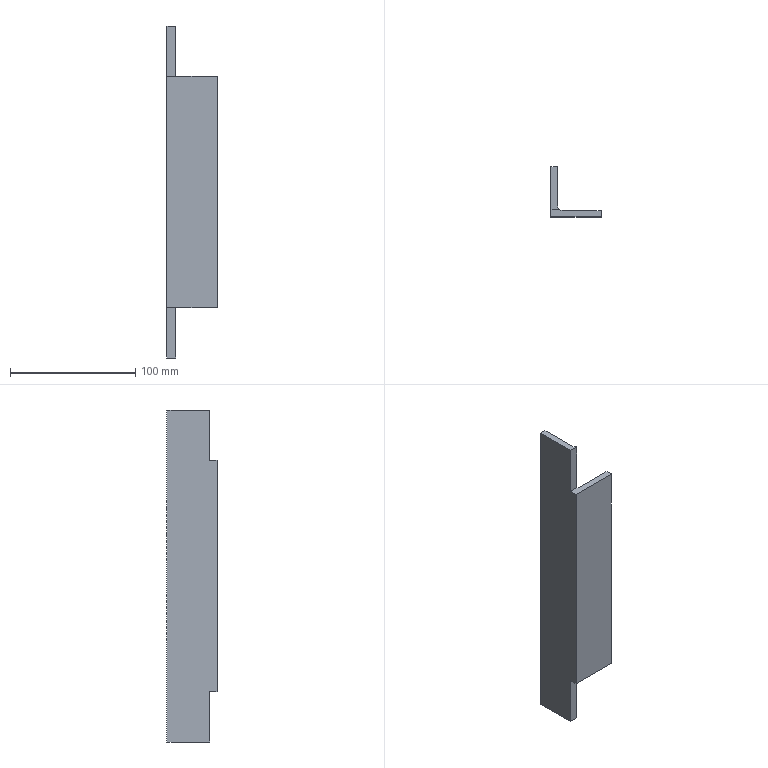Part | NX | features BREP 1 | 1 solid | 13 faces | box 40 x 40 x 265 mm | volume 84160 mm3 | plane 12 | cylinder 1 | commonest cylinder face diameters 10 x1
STEP:
#1=CARTESIAN_POINT('',(40.,5.,92.5));
#2=VERTEX_POINT('',#1);
#3=CARTESIAN_POINT('',(40.,5.,-92.5));
#4=VERTEX_POINT('',#3);
#5=CARTESIAN_POINT('',(40.,5.,132.5));
#6=DIRECTION('',(0.,0.,-1.));
#7=VECTOR('',#6,1000.);
#8=LINE('',#5,#7);
#9=EDGE_CURVE('',#2,#4,#8,.T.);
#10=ORIENTED_EDGE('',*,*,#9,.F.);
#11=CARTESIAN_POINT('',(40.,0.,92.5));
#12=VERTEX_POINT('',#11);
#13=CARTESIAN_POINT('',(40.,0.,92.5));
#14=DIRECTION('',(0.,-1.,0.));
#15=VECTOR('',#14,1000.);
#16=LINE('',#13,#15);
#17=EDGE_CURVE('',#2,#12,#16,.T.);
#18=ORIENTED_EDGE('',*,*,#17,.T.);
#19=CARTESIAN_POINT('',(40.,0.,-92.5));
#20=VERTEX_POINT('',#19);
#21=CARTESIAN_POINT('',(40.,0.,132.5));
#22=DIRECTION('',(0.,0.,-1.));
#23=VECTOR('',#22,1000.);
#24=LINE('',#21,#23);
#25=EDGE_CURVE('',#12,#20,#24,.T.);
#26=ORIENTED_EDGE('',*,*,#25,.T.);
#27=CARTESIAN_POINT('',(40.,0.,-92.5));
#28=DIRECTION('',(0.,1.,0.));
#29=VECTOR('',#28,1000.);
#30=LINE('',#27,#29);
#31=EDGE_CURVE('',#20,#4,#30,.T.);
#32=ORIENTED_EDGE('',*,*,#31,.T.);
#33=EDGE_LOOP('',(#10,#18,#26,#32));
#34=FACE_BOUND('',#33,.T.);
#35=CARTESIAN_POINT('',(40.,5.,132.5));
#36=DIRECTION('',(-1.,0.,0.));
#37=DIRECTION('',(0.,0.,-1.));
#38=AXIS2_PLACEMENT_3D('',#35,#36,#37);
#39=PLANE('',#38);
#40=ADVANCED_FACE('',(#34),#39,.F.);
#41=CARTESIAN_POINT('',(10.,5.,92.5));
#42=VERTEX_POINT('',#41);
#43=CARTESIAN_POINT('',(10.,5.,-92.5));
#44=VERTEX_POINT('',#43);
#45=CARTESIAN_POINT('',(10.,5.,132.5));
#46=DIRECTION('',(0.,0.,-1.));
#47=VECTOR('',#46,1000.);
#48=LINE('',#45,#47);
#49=EDGE_CURVE('',#42,#44,#48,.T.);
#50=ORIENTED_EDGE('',*,*,#49,.F.);
#51=CARTESIAN_POINT('',(10.,5.,92.5));
#52=DIRECTION('',(1.,0.,0.));
#53=VECTOR('',#52,1000.);
#54=LINE('',#51,#53);
#55=EDGE_CURVE('',#42,#2,#54,.T.);
#56=ORIENTED_EDGE('',*,*,#55,.T.);
#57=ORIENTED_EDGE('',*,*,#9,.T.);
#58=CARTESIAN_POINT('',(10.,5.,-92.5));
#59=DIRECTION('',(-1.,0.,0.));
#60=VECTOR('',#59,1000.);
#61=LINE('',#58,#60);
#62=EDGE_CURVE('',#4,#44,#61,.T.);
#63=ORIENTED_EDGE('',*,*,#62,.T.);
#64=EDGE_LOOP('',(#50,#56,#57,#63));
#65=FACE_BOUND('',#64,.T.);
#66=CARTESIAN_POINT('',(10.,5.,132.5));
#67=DIRECTION('',(0.,-1.,0.));
#68=DIRECTION('',(0.,0.,1.));
#69=AXIS2_PLACEMENT_3D('',#66,#67,#68);
#70=PLANE('',#69);
#71=ADVANCED_FACE('',(#65),#70,.F.);
#72=CARTESIAN_POINT('',(7.,6.,132.5));
#73=VERTEX_POINT('',#72);
#74=CARTESIAN_POINT('',(7.,6.,92.5));
#75=VERTEX_POINT('',#74);
#76=CARTESIAN_POINT('',(7.,6.,132.5));
#77=DIRECTION('',(0.,0.,-1.));
#78=VECTOR('',#77,1000.);
#79=LINE('',#76,#78);
#80=EDGE_CURVE('',#73,#75,#79,.T.);
#81=ORIENTED_EDGE('',*,*,#80,.T.);
#82=CARTESIAN_POINT('',(10.,10.,92.5));
#83=DIRECTION('',(0.,0.,1.));
#84=DIRECTION('',(-1.,0.,0.));
#85=AXIS2_PLACEMENT_3D('',#82,#83,#84);
#86=CIRCLE('',#85,5.);
#87=EDGE_CURVE('',#75,#42,#86,.T.);
#88=ORIENTED_EDGE('',*,*,#87,.T.);
#89=ORIENTED_EDGE('',*,*,#49,.T.);
#90=CARTESIAN_POINT('',(7.,6.,-92.5));
#91=VERTEX_POINT('',#90);
#92=CARTESIAN_POINT('',(10.,10.,-92.5));
#93=DIRECTION('',(0.,0.,-1.));
#94=DIRECTION('',(1.,0.,0.));
#95=AXIS2_PLACEMENT_3D('',#92,#93,#94);
#96=CIRCLE('',#95,5.);
#97=EDGE_CURVE('',#44,#91,#96,.T.);
#98=ORIENTED_EDGE('',*,*,#97,.T.);
#99=CARTESIAN_POINT('',(7.,6.,-132.5));
#100=VERTEX_POINT('',#99);
#101=CARTESIAN_POINT('',(7.,6.,132.5));
#102=DIRECTION('',(0.,0.,-1.));
#103=VECTOR('',#102,1000.);
#104=LINE('',#101,#103);
#105=EDGE_CURVE('',#91,#100,#104,.T.);
#106=ORIENTED_EDGE('',*,*,#105,.T.);
#107=CARTESIAN_POINT('',(5.,10.,-132.5));
#108=VERTEX_POINT('',#107);
#109=CARTESIAN_POINT('',(10.,10.,-132.5));
#110=DIRECTION('',(0.,0.,-1.));
#111=DIRECTION('',(1.,0.,0.));
#112=AXIS2_PLACEMENT_3D('',#109,#110,#111);
#113=CIRCLE('',#112,5.);
#114=EDGE_CURVE('',#100,#108,#113,.T.);
#115=ORIENTED_EDGE('',*,*,#114,.T.);
#116=CARTESIAN_POINT('',(5.,10.,132.5));
#117=VERTEX_POINT('',#116);
#118=CARTESIAN_POINT('',(5.,10.,132.5));
#119=DIRECTION('',(0.,0.,-1.));
#120=VECTOR('',#119,1000.);
#121=LINE('',#118,#120);
#122=EDGE_CURVE('',#117,#108,#121,.T.);
#123=ORIENTED_EDGE('',*,*,#122,.F.);
#124=CARTESIAN_POINT('',(10.,10.,132.5));
#125=DIRECTION('',(0.,0.,-1.));
#126=DIRECTION('',(1.,0.,0.));
#127=AXIS2_PLACEMENT_3D('',#124,#125,#126);
#128=CIRCLE('',#127,5.);
#129=EDGE_CURVE('',#73,#117,#128,.T.);
#130=ORIENTED_EDGE('',*,*,#129,.F.);
#131=EDGE_LOOP('',(#81,#88,#89,#98,#106,#115,#123,#130));
#132=FACE_BOUND('',#131,.T.);
#133=CARTESIAN_POINT('',(10.,10.,132.5));
#134=DIRECTION('',(0.,0.,-1.));
#135=DIRECTION('',(1.,0.,0.));
#136=AXIS2_PLACEMENT_3D('',#133,#134,#135);
#137=CYLINDRICAL_SURFACE('',#136,5.);
#138=ADVANCED_FACE('',(#132),#137,.F.);
#139=CARTESIAN_POINT('',(5.,40.,-132.5));
#140=VERTEX_POINT('',#139);
#141=CARTESIAN_POINT('',(5.,40.,-132.5));
#142=DIRECTION('',(0.,1.,0.));
#143=VECTOR('',#142,1000.);
#144=LINE('',#141,#143);
#145=EDGE_CURVE('',#108,#140,#144,.T.);
#146=ORIENTED_EDGE('',*,*,#145,.T.);
#147=CARTESIAN_POINT('',(5.,40.,132.5));
#148=VERTEX_POINT('',#147);
#149=CARTESIAN_POINT('',(5.,40.,132.5));
#150=DIRECTION('',(0.,0.,-1.));
#151=VECTOR('',#150,1000.);
#152=LINE('',#149,#151);
#153=EDGE_CURVE('',#148,#140,#152,.T.);
#154=ORIENTED_EDGE('',*,*,#153,.F.);
#155=CARTESIAN_POINT('',(5.,40.,132.5));
#156=DIRECTION('',(0.,1.,0.));
#157=VECTOR('',#156,1000.);
#158=LINE('',#155,#157);
#159=EDGE_CURVE('',#117,#148,#158,.T.);
#160=ORIENTED_EDGE('',*,*,#159,.F.);
#161=ORIENTED_EDGE('',*,*,#122,.T.);
#162=EDGE_LOOP('',(#146,#154,#160,#161));
#163=FACE_BOUND('',#162,.T.);
#164=CARTESIAN_POINT('',(5.,40.,132.5));
#165=DIRECTION('',(-1.,0.,0.));
#166=DIRECTION('',(0.,0.,-1.));
#167=AXIS2_PLACEMENT_3D('',#164,#165,#166);
#168=PLANE('',#167);
#169=ADVANCED_FACE('',(#163),#168,.F.);
#170=CARTESIAN_POINT('',(0.,40.,-132.5));
#171=VERTEX_POINT('',#170);
#172=CARTESIAN_POINT('',(0.,40.,-132.5));
#173=DIRECTION('',(-1.,0.,0.));
#174=VECTOR('',#173,1000.);
#175=LINE('',#172,#174);
#176=EDGE_CURVE('',#140,#171,#175,.T.);
#177=ORIENTED_EDGE('',*,*,#176,.T.);
#178=CARTESIAN_POINT('',(0.,40.,132.5));
#179=VERTEX_POINT('',#178);
#180=CARTESIAN_POINT('',(0.,40.,132.5));
#181=DIRECTION('',(0.,0.,-1.));
#182=VECTOR('',#181,1000.);
#183=LINE('',#180,#182);
#184=EDGE_CURVE('',#179,#171,#183,.T.);
#185=ORIENTED_EDGE('',*,*,#184,.F.);
#186=CARTESIAN_POINT('',(0.,40.,132.5));
#187=DIRECTION('',(-1.,0.,0.));
#188=VECTOR('',#187,1000.);
#189=LINE('',#186,#188);
#190=EDGE_CURVE('',#148,#179,#189,.T.);
#191=ORIENTED_EDGE('',*,*,#190,.F.);
#192=ORIENTED_EDGE('',*,*,#153,.T.);
#193=EDGE_LOOP('',(#177,#185,#191,#192));
#194=FACE_BOUND('',#193,.T.);
#195=CARTESIAN_POINT('',(0.,40.,132.5));
#196=DIRECTION('',(0.,-1.,0.));
#197=DIRECTION('',(0.,0.,1.));
#198=AXIS2_PLACEMENT_3D('',#195,#196,#197);
#199=PLANE('',#198);
#200=ADVANCED_FACE('',(#194),#199,.F.);
#201=CARTESIAN_POINT('',(0.,0.,92.5));
#202=VERTEX_POINT('',#201);
#203=CARTESIAN_POINT('',(0.,0.,-92.5));
#204=VERTEX_POINT('',#203);
#205=CARTESIAN_POINT('',(0.,0.,132.5));
#206=DIRECTION('',(0.,0.,-1.));
#207=VECTOR('',#206,1000.);
#208=LINE('',#205,#207);
#209=EDGE_CURVE('',#202,#204,#208,.T.);
#210=ORIENTED_EDGE('',*,*,#209,.F.);
#211=CARTESIAN_POINT('',(0.,6.,92.5));
#212=VERTEX_POINT('',#211);
#213=CARTESIAN_POINT('',(0.,0.,92.5));
#214=DIRECTION('',(0.,-1.,0.));
#215=VECTOR('',#214,1000.);
#216=LINE('',#213,#215);
#217=EDGE_CURVE('',#212,#202,#216,.T.);
#218=ORIENTED_EDGE('',*,*,#217,.F.);
#219=CARTESIAN_POINT('',(0.,6.,132.5));
#220=VERTEX_POINT('',#219);
#221=CARTESIAN_POINT('',(0.,6.,132.5));
#222=DIRECTION('',(0.,0.,-1.));
#223=VECTOR('',#222,1000.);
#224=LINE('',#221,#223);
#225=EDGE_CURVE('',#220,#212,#224,.T.);
#226=ORIENTED_EDGE('',*,*,#225,.F.);
#227=CARTESIAN_POINT('',(0.,0.,132.5));
#228=DIRECTION('',(0.,-1.,0.));
#229=VECTOR('',#228,1000.);
#230=LINE('',#227,#229);
#231=EDGE_CURVE('',#179,#220,#230,.T.);
#232=ORIENTED_EDGE('',*,*,#231,.F.);
#233=ORIENTED_EDGE('',*,*,#184,.T.);
#234=CARTESIAN_POINT('',(0.,6.,-132.5));
#235=VERTEX_POINT('',#234);
#236=CARTESIAN_POINT('',(0.,0.,-132.5));
#237=DIRECTION('',(0.,-1.,0.));
#238=VECTOR('',#237,1000.);
#239=LINE('',#236,#238);
#240=EDGE_CURVE('',#171,#235,#239,.T.);
#241=ORIENTED_EDGE('',*,*,#240,.T.);
#242=CARTESIAN_POINT('',(0.,6.,-92.5));
#243=VERTEX_POINT('',#242);
#244=CARTESIAN_POINT('',(0.,6.,-132.5));
#245=DIRECTION('',(0.,0.,-1.));
#246=VECTOR('',#245,1000.);
#247=LINE('',#244,#246);
#248=EDGE_CURVE('',#243,#235,#247,.T.);
#249=ORIENTED_EDGE('',*,*,#248,.F.);
#250=CARTESIAN_POINT('',(0.,0.,-92.5));
#251=DIRECTION('',(0.,1.,0.));
#252=VECTOR('',#251,1000.);
#253=LINE('',#250,#252);
#254=EDGE_CURVE('',#204,#243,#253,.T.);
#255=ORIENTED_EDGE('',*,*,#254,.F.);
#256=EDGE_LOOP('',(#210,#218,#226,#232,#233,#241,#249,#255));
#257=FACE_BOUND('',#256,.T.);
#258=CARTESIAN_POINT('',(0.,0.,132.5));
#259=DIRECTION('',(1.,0.,0.));
#260=DIRECTION('',(0.,0.,1.));
#261=AXIS2_PLACEMENT_3D('',#258,#259,#260);
#262=PLANE('',#261);
#263=ADVANCED_FACE('',(#257),#262,.F.);
#264=ORIENTED_EDGE('',*,*,#25,.F.);
#265=CARTESIAN_POINT('',(40.,0.,92.5));
#266=DIRECTION('',(-1.,0.,0.));
#267=VECTOR('',#266,1000.);
#268=LINE('',#265,#267);
#269=EDGE_CURVE('',#12,#202,#268,.T.);
#270=ORIENTED_EDGE('',*,*,#269,.T.);
#271=ORIENTED_EDGE('',*,*,#209,.T.);
#272=CARTESIAN_POINT('',(40.,0.,-92.5));
#273=DIRECTION('',(-1.,0.,0.));
#274=VECTOR('',#273,1000.);
#275=LINE('',#272,#274);
#276=EDGE_CURVE('',#20,#204,#275,.T.);
#277=ORIENTED_EDGE('',*,*,#276,.F.);
#278=EDGE_LOOP('',(#264,#270,#271,#277));
#279=FACE_BOUND('',#278,.T.);
#280=CARTESIAN_POINT('',(40.,0.,132.5));
#281=DIRECTION('',(0.,1.,0.));
#282=DIRECTION('',(0.,0.,-1.));
#283=AXIS2_PLACEMENT_3D('',#280,#281,#282);
#284=PLANE('',#283);
#285=ADVANCED_FACE('',(#279),#284,.F.);
#286=CARTESIAN_POINT('',(10.,6.,132.5));
#287=DIRECTION('',(-1.,0.,0.));
#288=VECTOR('',#287,1000.);
#289=LINE('',#286,#288);
#290=EDGE_CURVE('',#73,#220,#289,.T.);
#291=ORIENTED_EDGE('',*,*,#290,.F.);
#292=ORIENTED_EDGE('',*,*,#129,.T.);
#293=ORIENTED_EDGE('',*,*,#159,.T.);
#294=ORIENTED_EDGE('',*,*,#190,.T.);
#295=ORIENTED_EDGE('',*,*,#231,.T.);
#296=EDGE_LOOP('',(#291,#292,#293,#294,#295));
#297=FACE_BOUND('',#296,.T.);
#298=CARTESIAN_POINT('',(10.,10.,132.5));
#299=DIRECTION('',(0.,0.,1.));
#300=DIRECTION('',(-1.,0.,0.));
#301=AXIS2_PLACEMENT_3D('',#298,#299,#300);
#302=PLANE('',#301);
#303=ADVANCED_FACE('',(#297),#302,.T.);
#304=ORIENTED_EDGE('',*,*,#114,.F.);
#305=CARTESIAN_POINT('',(10.,6.,-132.5));
#306=DIRECTION('',(-1.,0.,0.));
#307=VECTOR('',#306,1000.);
#308=LINE('',#305,#307);
#309=EDGE_CURVE('',#100,#235,#308,.T.);
#310=ORIENTED_EDGE('',*,*,#309,.T.);
#311=ORIENTED_EDGE('',*,*,#240,.F.);
#312=ORIENTED_EDGE('',*,*,#176,.F.);
#313=ORIENTED_EDGE('',*,*,#145,.F.);
#314=EDGE_LOOP('',(#304,#310,#311,#312,#313));
#315=FACE_BOUND('',#314,.T.);
#316=CARTESIAN_POINT('',(10.,10.,-132.5));
#317=DIRECTION('',(0.,0.,1.));
#318=DIRECTION('',(-1.,0.,0.));
#319=AXIS2_PLACEMENT_3D('',#316,#317,#318);
#320=PLANE('',#319);
#321=ADVANCED_FACE('',(#315),#320,.F.);
#322=ORIENTED_EDGE('',*,*,#31,.F.);
#323=ORIENTED_EDGE('',*,*,#276,.T.);
#324=ORIENTED_EDGE('',*,*,#254,.T.);
#325=CARTESIAN_POINT('',(40.,6.,-92.5));
#326=DIRECTION('',(-1.,0.,0.));
#327=VECTOR('',#326,1000.);
#328=LINE('',#325,#327);
#329=EDGE_CURVE('',#91,#243,#328,.T.);
#330=ORIENTED_EDGE('',*,*,#329,.F.);
#331=ORIENTED_EDGE('',*,*,#97,.F.);
#332=ORIENTED_EDGE('',*,*,#62,.F.);
#333=EDGE_LOOP('',(#322,#323,#324,#330,#331,#332));
#334=FACE_BOUND('',#333,.T.);
#335=CARTESIAN_POINT('',(40.,0.,-92.5));
#336=DIRECTION('',(0.,0.,1.));
#337=DIRECTION('',(-1.,0.,0.));
#338=AXIS2_PLACEMENT_3D('',#335,#336,#337);
#339=PLANE('',#338);
#340=ADVANCED_FACE('',(#334),#339,.F.);
#341=ORIENTED_EDGE('',*,*,#329,.T.);
#342=ORIENTED_EDGE('',*,*,#248,.T.);
#343=ORIENTED_EDGE('',*,*,#309,.F.);
#344=ORIENTED_EDGE('',*,*,#105,.F.);
#345=EDGE_LOOP('',(#341,#342,#343,#344));
#346=FACE_BOUND('',#345,.T.);
#347=CARTESIAN_POINT('',(40.,6.,-132.5));
#348=DIRECTION('',(0.,1.,0.));
#349=DIRECTION('',(0.,0.,-1.));
#350=AXIS2_PLACEMENT_3D('',#347,#348,#349);
#351=PLANE('',#350);
#352=ADVANCED_FACE('',(#346),#351,.F.);
#353=ORIENTED_EDGE('',*,*,#87,.F.);
#354=CARTESIAN_POINT('',(40.,6.,92.5));
#355=DIRECTION('',(-1.,0.,0.));
#356=VECTOR('',#355,1000.);
#357=LINE('',#354,#356);
#358=EDGE_CURVE('',#75,#212,#357,.T.);
#359=ORIENTED_EDGE('',*,*,#358,.T.);
#360=ORIENTED_EDGE('',*,*,#217,.T.);
#361=ORIENTED_EDGE('',*,*,#269,.F.);
#362=ORIENTED_EDGE('',*,*,#17,.F.);
#363=ORIENTED_EDGE('',*,*,#55,.F.);
#364=EDGE_LOOP('',(#353,#359,#360,#361,#362,#363));
#365=FACE_BOUND('',#364,.T.);
#366=CARTESIAN_POINT('',(40.,0.,92.5));
#367=DIRECTION('',(0.,0.,-1.));
#368=DIRECTION('',(1.,0.,0.));
#369=AXIS2_PLACEMENT_3D('',#366,#367,#368);
#370=PLANE('',#369);
#371=ADVANCED_FACE('',(#365),#370,.F.);
#372=ORIENTED_EDGE('',*,*,#290,.T.);
#373=ORIENTED_EDGE('',*,*,#225,.T.);
#374=ORIENTED_EDGE('',*,*,#358,.F.);
#375=ORIENTED_EDGE('',*,*,#80,.F.);
#376=EDGE_LOOP('',(#372,#373,#374,#375));
#377=FACE_BOUND('',#376,.T.);
#378=CARTESIAN_POINT('',(40.,6.,132.5));
#379=DIRECTION('',(0.,1.,0.));
#380=DIRECTION('',(0.,0.,-1.));
#381=AXIS2_PLACEMENT_3D('',#378,#379,#380);
#382=PLANE('',#381);
#383=ADVANCED_FACE('',(#377),#382,.F.);
#384=CLOSED_SHELL('',(#40,#71,#138,#169,#200,#263,#285,#303,#321,#340,#352,#371,#383));
#385=MANIFOLD_SOLID_BREP('',#384);
#386=(LENGTH_UNIT()NAMED_UNIT(*)SI_UNIT(.MILLI.,.METRE.));
#387=UNCERTAINTY_MEASURE_WITH_UNIT(LENGTH_MEASURE(0.00001),#386,'','');
#388=(NAMED_UNIT(*)PLANE_ANGLE_UNIT()SI_UNIT($,.RADIAN.));
#389=(NAMED_UNIT(*)SI_UNIT($,.STERADIAN.)SOLID_ANGLE_UNIT());
#390=(GEOMETRIC_REPRESENTATION_CONTEXT(3)GLOBAL_UNCERTAINTY_ASSIGNED_CONTEXT((#387))GLOBAL_UNIT_ASSIGNED_CONTEXT((#386,#388,#389))REPRESENTATION_CONTEXT('',''));
#391=ADVANCED_BREP_SHAPE_REPRESENTATION('',(#385),#390);